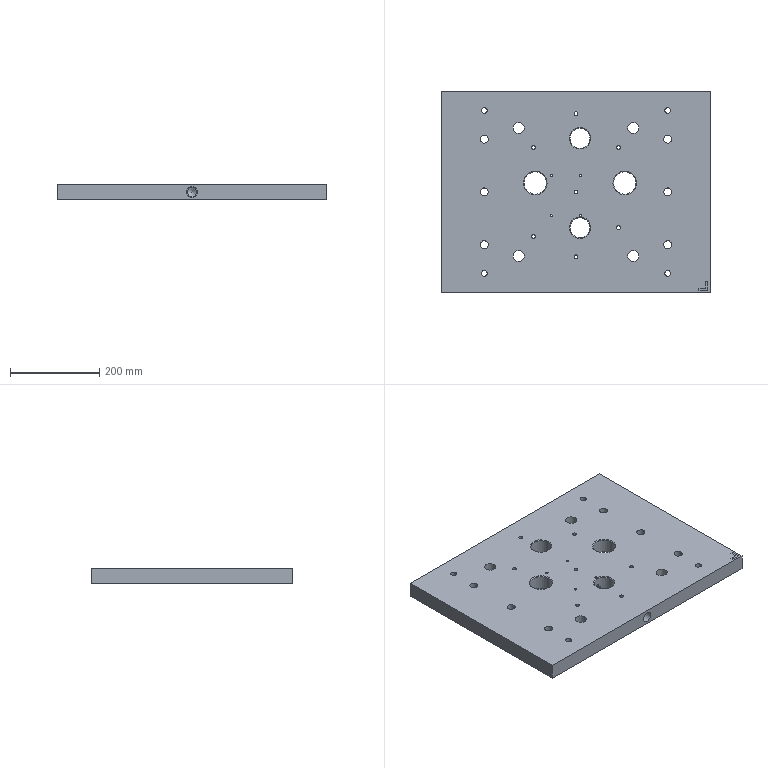Part | STEP file | BD | 1 solid | 167 faces | box 600 x 450 x 35 mm | volume 8925184 mm3 | cylinder 84 | plane 69 | cone 14 | commonest cylinder face diameters 6 x16 5 x8 8.5 x7 14 x7 18 x6 26 x6